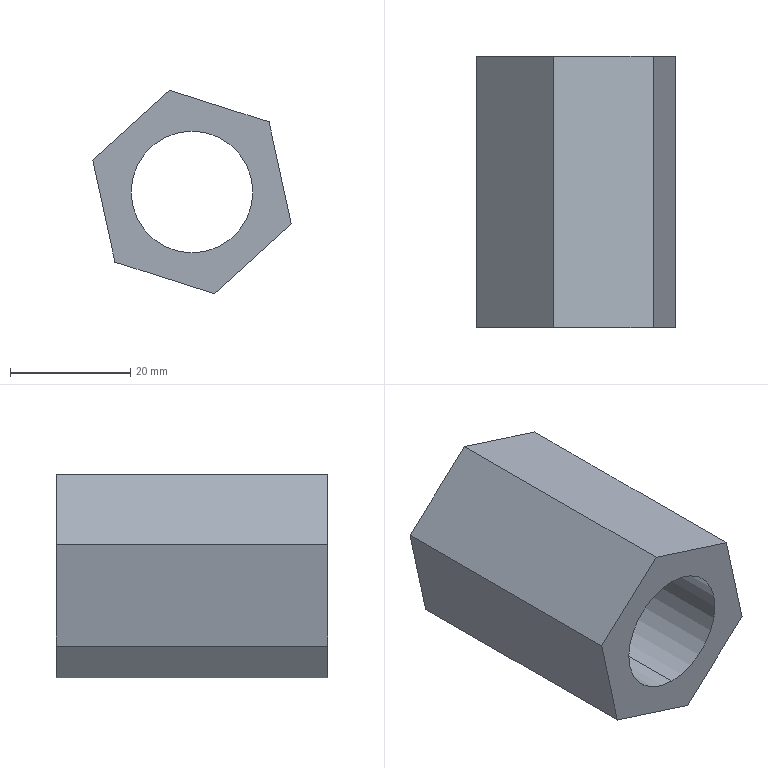Part | STEP file | 1 solid | 10 faces | box 32.935 x 45 x 33.783 mm | volume 20505 mm3 | plane 8 | cylinder 2 | commonest cylinder face diameters 20.209 x2
STEP:
#1=CARTESIAN_POINT('',(0.,0.,0.));
#2=DIRECTION('',(0.,0.,1.));
#3=DIRECTION('',(1.,0.,0.));
#4=AXIS2_PLACEMENT_3D('',#1,#2,#3);
#5=CARTESIAN_POINT('',(340.649,189.014,256.211));
#6=VERTEX_POINT('',#5);
#7=CARTESIAN_POINT('',(340.649,234.014,256.211));
#8=VERTEX_POINT('',#7);
#9=CARTESIAN_POINT('',(340.649,189.014,256.211));
#10=DIRECTION('',(0.,1.,0.));
#11=VECTOR('',#10,1.);
#12=LINE('',#9,#11);
#13=CARTESIAN_POINT('',(340.649,189.014,246.106));
#14=DIRECTION('',(0.,1.,0.));
#15=DIRECTION('',(0.,0.,1.));
#16=AXIS2_PLACEMENT_3D('',#13,#14,#15);
#17=CYLINDRICAL_SURFACE('',#16,10.105);
#18=CARTESIAN_POINT('',(6.283,0.));
#19=DIRECTION('',(0.,1.));
#20=VECTOR('',#19,1.);
#21=LINE('',#18,#20);
#22=(GEOMETRIC_REPRESENTATION_CONTEXT(2)PARAMETRIC_REPRESENTATION_CONTEXT()REPRESENTATION_CONTEXT('',''));
#23=DEFINITIONAL_REPRESENTATION('',(#21),#22);
#24=PCURVE('',#17,#23);
#25=CARTESIAN_POINT('',(340.649,189.014,246.106));
#26=DIRECTION('',(0.,1.,0.));
#27=DIRECTION('',(0.,0.,1.));
#28=AXIS2_PLACEMENT_3D('',#25,#26,#27);
#29=CYLINDRICAL_SURFACE('',#28,10.105);
#30=CARTESIAN_POINT('',(0.,0.));
#31=DIRECTION('',(0.,1.));
#32=VECTOR('',#31,1.);
#33=LINE('',#30,#32);
#34=(GEOMETRIC_REPRESENTATION_CONTEXT(2)PARAMETRIC_REPRESENTATION_CONTEXT()REPRESENTATION_CONTEXT('',''));
#35=DEFINITIONAL_REPRESENTATION('',(#33),#34);
#36=PCURVE('',#29,#35);
#37=SURFACE_CURVE('',#12,(#24,#36),.PCURVE_S1.);
#38=EDGE_CURVE('',#6,#8,#37,.T.);
#39=ORIENTED_EDGE('',*,*,#38,.T.);
#40=CARTESIAN_POINT('',(340.649,234.014,236.001));
#41=VERTEX_POINT('',#40);
#42=CARTESIAN_POINT('',(340.649,234.014,246.106));
#43=DIRECTION('',(0.,-1.,0.));
#44=DIRECTION('',(0.,0.,-1.));
#45=AXIS2_PLACEMENT_3D('',#42,#43,#44);
#46=CIRCLE('',#45,10.105);
#47=CARTESIAN_POINT('',(9.425,45.));
#48=DIRECTION('',(-1.,0.));
#49=VECTOR('',#48,1.);
#50=LINE('',#47,#49);
#51=(GEOMETRIC_REPRESENTATION_CONTEXT(2)PARAMETRIC_REPRESENTATION_CONTEXT()REPRESENTATION_CONTEXT('',''));
#52=DEFINITIONAL_REPRESENTATION('',(#50),#51);
#53=PCURVE('',#17,#52);
#54=CARTESIAN_POINT('',(0.,234.014,0.));
#55=DIRECTION('',(0.,-1.,0.));
#56=DIRECTION('',(0.,0.,-1.));
#57=AXIS2_PLACEMENT_3D('',#54,#55,#56);
#58=PLANE('',#57);
#59=CARTESIAN_POINT('',(-246.106,340.649));
#60=DIRECTION('',(1.,0.));
#61=AXIS2_PLACEMENT_2D('',#59,#60);
#62=CIRCLE('',#61,10.105);
#63=(GEOMETRIC_REPRESENTATION_CONTEXT(2)PARAMETRIC_REPRESENTATION_CONTEXT()REPRESENTATION_CONTEXT('',''));
#64=DEFINITIONAL_REPRESENTATION('',(#62),#63);
#65=PCURVE('',#58,#64);
#66=SURFACE_CURVE('',#46,(#53,#65),.PCURVE_S1.);
#67=EDGE_CURVE('',#8,#41,#66,.T.);
#68=ORIENTED_EDGE('',*,*,#67,.T.);
#69=CARTESIAN_POINT('',(340.649,189.014,236.001));
#70=VERTEX_POINT('',#69);
#71=CARTESIAN_POINT('',(340.649,189.014,236.001));
#72=DIRECTION('',(0.,1.,0.));
#73=VECTOR('',#72,1.);
#74=LINE('',#71,#73);
#75=CARTESIAN_POINT('',(3.142,0.));
#76=DIRECTION('',(0.,1.));
#77=VECTOR('',#76,1.);
#78=LINE('',#75,#77);
#79=(GEOMETRIC_REPRESENTATION_CONTEXT(2)PARAMETRIC_REPRESENTATION_CONTEXT()REPRESENTATION_CONTEXT('',''));
#80=DEFINITIONAL_REPRESENTATION('',(#78),#79);
#81=PCURVE('',#17,#80);
#82=CARTESIAN_POINT('',(3.142,0.));
#83=DIRECTION('',(0.,1.));
#84=VECTOR('',#83,1.);
#85=LINE('',#82,#84);
#86=(GEOMETRIC_REPRESENTATION_CONTEXT(2)PARAMETRIC_REPRESENTATION_CONTEXT()REPRESENTATION_CONTEXT('',''));
#87=DEFINITIONAL_REPRESENTATION('',(#85),#86);
#88=PCURVE('',#29,#87);
#89=SURFACE_CURVE('',#74,(#81,#88),.PCURVE_S1.);
#90=EDGE_CURVE('',#70,#41,#89,.T.);
#91=ORIENTED_EDGE('',*,*,#90,.F.);
#92=CARTESIAN_POINT('',(340.649,189.014,246.106));
#93=DIRECTION('',(0.,-1.,0.));
#94=DIRECTION('',(0.,0.,-1.));
#95=AXIS2_PLACEMENT_3D('',#92,#93,#94);
#96=CIRCLE('',#95,10.105);
#97=CARTESIAN_POINT('',(9.425,0.));
#98=DIRECTION('',(-1.,0.));
#99=VECTOR('',#98,1.);
#100=LINE('',#97,#99);
#101=(GEOMETRIC_REPRESENTATION_CONTEXT(2)PARAMETRIC_REPRESENTATION_CONTEXT()REPRESENTATION_CONTEXT('',''));
#102=DEFINITIONAL_REPRESENTATION('',(#100),#101);
#103=PCURVE('',#17,#102);
#104=CARTESIAN_POINT('',(0.,189.014,0.));
#105=DIRECTION('',(0.,-1.,0.));
#106=DIRECTION('',(0.,0.,-1.));
#107=AXIS2_PLACEMENT_3D('',#104,#105,#106);
#108=PLANE('',#107);
#109=CARTESIAN_POINT('',(-246.106,340.649));
#110=DIRECTION('',(1.,0.));
#111=AXIS2_PLACEMENT_2D('',#109,#110);
#112=CIRCLE('',#111,10.105);
#113=(GEOMETRIC_REPRESENTATION_CONTEXT(2)PARAMETRIC_REPRESENTATION_CONTEXT()REPRESENTATION_CONTEXT('',''));
#114=DEFINITIONAL_REPRESENTATION('',(#112),#113);
#115=PCURVE('',#108,#114);
#116=SURFACE_CURVE('',#96,(#103,#115),.PCURVE_S1.);
#117=EDGE_CURVE('',#6,#70,#116,.T.);
#118=ORIENTED_EDGE('',*,*,#117,.F.);
#119=EDGE_LOOP('',(#39,#68,#91,#118));
#120=FACE_BOUND('',#119,.F.);
#121=ADVANCED_FACE('',(#120),#17,.F.);
#122=CARTESIAN_POINT('',(357.116,189.014,240.846));
#123=VERTEX_POINT('',#122);
#124=CARTESIAN_POINT('',(353.438,189.014,257.737));
#125=VERTEX_POINT('',#124);
#126=CARTESIAN_POINT('',(357.116,189.014,240.846));
#127=DIRECTION('',(-0.2128,0.,0.9771));
#128=VECTOR('',#127,1.);
#129=LINE('',#126,#128);
#130=CARTESIAN_POINT('',(-240.846,357.116));
#131=DIRECTION('',(-0.9771,-0.2128));
#132=VECTOR('',#131,1.);
#133=LINE('',#130,#132);
#134=(GEOMETRIC_REPRESENTATION_CONTEXT(2)PARAMETRIC_REPRESENTATION_CONTEXT()REPRESENTATION_CONTEXT('',''));
#135=DEFINITIONAL_REPRESENTATION('',(#133),#134);
#136=PCURVE('',#108,#135);
#137=CARTESIAN_POINT('',(357.116,189.014,240.846));
#138=DIRECTION('',(-0.9771,0.,-0.2128));
#139=DIRECTION('',(-0.2128,0.,0.9771));
#140=AXIS2_PLACEMENT_3D('',#137,#138,#139);
#141=PLANE('',#140);
#142=CARTESIAN_POINT('',(0.,0.));
#143=DIRECTION('',(1.,0.));
#144=VECTOR('',#143,1.);
#145=LINE('',#142,#144);
#146=(GEOMETRIC_REPRESENTATION_CONTEXT(2)PARAMETRIC_REPRESENTATION_CONTEXT()REPRESENTATION_CONTEXT('',''));
#147=DEFINITIONAL_REPRESENTATION('',(#145),#146);
#148=PCURVE('',#141,#147);
#149=SURFACE_CURVE('',#129,(#136,#148),.PCURVE_S1.);
#150=EDGE_CURVE('',#123,#125,#149,.T.);
#151=ORIENTED_EDGE('',*,*,#150,.T.);
#152=CARTESIAN_POINT('',(336.97,189.014,262.997));
#153=VERTEX_POINT('',#152);
#154=CARTESIAN_POINT('',(353.438,189.014,257.737));
#155=DIRECTION('',(-0.9526,0.,0.3043));
#156=VECTOR('',#155,1.);
#157=LINE('',#154,#156);
#158=CARTESIAN_POINT('',(-257.737,353.438));
#159=DIRECTION('',(-0.3043,-0.9526));
#160=VECTOR('',#159,1.);
#161=LINE('',#158,#160);
#162=(GEOMETRIC_REPRESENTATION_CONTEXT(2)PARAMETRIC_REPRESENTATION_CONTEXT()REPRESENTATION_CONTEXT('',''));
#163=DEFINITIONAL_REPRESENTATION('',(#161),#162);
#164=PCURVE('',#108,#163);
#165=CARTESIAN_POINT('',(353.438,189.014,257.737));
#166=DIRECTION('',(-0.3043,0.,-0.9526));
#167=DIRECTION('',(-0.9526,0.,0.3043));
#168=AXIS2_PLACEMENT_3D('',#165,#166,#167);
#169=PLANE('',#168);
#170=CARTESIAN_POINT('',(0.,0.));
#171=DIRECTION('',(1.,0.));
#172=VECTOR('',#171,1.);
#173=LINE('',#170,#172);
#174=(GEOMETRIC_REPRESENTATION_CONTEXT(2)PARAMETRIC_REPRESENTATION_CONTEXT()REPRESENTATION_CONTEXT('',''));
#175=DEFINITIONAL_REPRESENTATION('',(#173),#174);
#176=PCURVE('',#169,#175);
#177=SURFACE_CURVE('',#157,(#164,#176),.PCURVE_S1.);
#178=EDGE_CURVE('',#125,#153,#177,.T.);
#179=ORIENTED_EDGE('',*,*,#178,.T.);
#180=CARTESIAN_POINT('',(324.181,189.014,251.366));
#181=VERTEX_POINT('',#180);
#182=CARTESIAN_POINT('',(336.97,189.014,262.997));
#183=DIRECTION('',(-0.7398,0.,-0.6728));
#184=VECTOR('',#183,1.);
#185=LINE('',#182,#184);
#186=CARTESIAN_POINT('',(-262.997,336.97));
#187=DIRECTION('',(0.6728,-0.7398));
#188=VECTOR('',#187,1.);
#189=LINE('',#186,#188);
#190=(GEOMETRIC_REPRESENTATION_CONTEXT(2)PARAMETRIC_REPRESENTATION_CONTEXT()REPRESENTATION_CONTEXT('',''));
#191=DEFINITIONAL_REPRESENTATION('',(#189),#190);
#192=PCURVE('',#108,#191);
#193=CARTESIAN_POINT('',(336.97,189.014,262.997));
#194=DIRECTION('',(0.6728,0.,-0.7398));
#195=DIRECTION('',(-0.7398,0.,-0.6728));
#196=AXIS2_PLACEMENT_3D('',#193,#194,#195);
#197=PLANE('',#196);
#198=CARTESIAN_POINT('',(0.,0.));
#199=DIRECTION('',(1.,0.));
#200=VECTOR('',#199,1.);
#201=LINE('',#198,#200);
#202=(GEOMETRIC_REPRESENTATION_CONTEXT(2)PARAMETRIC_REPRESENTATION_CONTEXT()REPRESENTATION_CONTEXT('',''));
#203=DEFINITIONAL_REPRESENTATION('',(#201),#202);
#204=PCURVE('',#197,#203);
#205=SURFACE_CURVE('',#185,(#192,#204),.PCURVE_S1.);
#206=EDGE_CURVE('',#153,#181,#205,.T.);
#207=ORIENTED_EDGE('',*,*,#206,.T.);
#208=CARTESIAN_POINT('',(327.859,189.014,234.474));
#209=VERTEX_POINT('',#208);
#210=CARTESIAN_POINT('',(324.181,189.014,251.366));
#211=DIRECTION('',(0.2128,0.,-0.9771));
#212=VECTOR('',#211,1.);
#213=LINE('',#210,#212);
#214=CARTESIAN_POINT('',(-251.366,324.181));
#215=DIRECTION('',(0.9771,0.2128));
#216=VECTOR('',#215,1.);
#217=LINE('',#214,#216);
#218=(GEOMETRIC_REPRESENTATION_CONTEXT(2)PARAMETRIC_REPRESENTATION_CONTEXT()REPRESENTATION_CONTEXT('',''));
#219=DEFINITIONAL_REPRESENTATION('',(#217),#218);
#220=PCURVE('',#108,#219);
#221=CARTESIAN_POINT('',(324.181,189.014,251.366));
#222=DIRECTION('',(0.9771,0.,0.2128));
#223=DIRECTION('',(0.2128,0.,-0.9771));
#224=AXIS2_PLACEMENT_3D('',#221,#222,#223);
#225=PLANE('',#224);
#226=CARTESIAN_POINT('',(0.,0.));
#227=DIRECTION('',(1.,0.));
#228=VECTOR('',#227,1.);
#229=LINE('',#226,#228);
#230=(GEOMETRIC_REPRESENTATION_CONTEXT(2)PARAMETRIC_REPRESENTATION_CONTEXT()REPRESENTATION_CONTEXT('',''));
#231=DEFINITIONAL_REPRESENTATION('',(#229),#230);
#232=PCURVE('',#225,#231);
#233=SURFACE_CURVE('',#213,(#220,#232),.PCURVE_S1.);
#234=EDGE_CURVE('',#181,#209,#233,.T.);
#235=ORIENTED_EDGE('',*,*,#234,.T.);
#236=CARTESIAN_POINT('',(344.327,189.014,229.214));
#237=VERTEX_POINT('',#236);
#238=CARTESIAN_POINT('',(327.859,189.014,234.474));
#239=DIRECTION('',(0.9526,0.,-0.3043));
#240=VECTOR('',#239,1.);
#241=LINE('',#238,#240);
#242=CARTESIAN_POINT('',(-234.474,327.859));
#243=DIRECTION('',(0.3043,0.9526));
#244=VECTOR('',#243,1.);
#245=LINE('',#242,#244);
#246=(GEOMETRIC_REPRESENTATION_CONTEXT(2)PARAMETRIC_REPRESENTATION_CONTEXT()REPRESENTATION_CONTEXT('',''));
#247=DEFINITIONAL_REPRESENTATION('',(#245),#246);
#248=PCURVE('',#108,#247);
#249=CARTESIAN_POINT('',(327.859,189.014,234.474));
#250=DIRECTION('',(0.3043,0.,0.9526));
#251=DIRECTION('',(0.9526,0.,-0.3043));
#252=AXIS2_PLACEMENT_3D('',#249,#250,#251);
#253=PLANE('',#252);
#254=CARTESIAN_POINT('',(0.,0.));
#255=DIRECTION('',(1.,0.));
#256=VECTOR('',#255,1.);
#257=LINE('',#254,#256);
#258=(GEOMETRIC_REPRESENTATION_CONTEXT(2)PARAMETRIC_REPRESENTATION_CONTEXT()REPRESENTATION_CONTEXT('',''));
#259=DEFINITIONAL_REPRESENTATION('',(#257),#258);
#260=PCURVE('',#253,#259);
#261=SURFACE_CURVE('',#241,(#248,#260),.PCURVE_S1.);
#262=EDGE_CURVE('',#209,#237,#261,.T.);
#263=ORIENTED_EDGE('',*,*,#262,.T.);
#264=CARTESIAN_POINT('',(344.327,189.014,229.214));
#265=DIRECTION('',(0.7398,0.,0.6728));
#266=VECTOR('',#265,1.);
#267=LINE('',#264,#266);
#268=CARTESIAN_POINT('',(-229.214,344.327));
#269=DIRECTION('',(-0.6728,0.7398));
#270=VECTOR('',#269,1.);
#271=LINE('',#268,#270);
#272=(GEOMETRIC_REPRESENTATION_CONTEXT(2)PARAMETRIC_REPRESENTATION_CONTEXT()REPRESENTATION_CONTEXT('',''));
#273=DEFINITIONAL_REPRESENTATION('',(#271),#272);
#274=PCURVE('',#108,#273);
#275=CARTESIAN_POINT('',(344.327,189.014,229.214));
#276=DIRECTION('',(-0.6728,0.,0.7398));
#277=DIRECTION('',(0.7398,0.,0.6728));
#278=AXIS2_PLACEMENT_3D('',#275,#276,#277);
#279=PLANE('',#278);
#280=CARTESIAN_POINT('',(0.,0.));
#281=DIRECTION('',(1.,0.));
#282=VECTOR('',#281,1.);
#283=LINE('',#280,#282);
#284=(GEOMETRIC_REPRESENTATION_CONTEXT(2)PARAMETRIC_REPRESENTATION_CONTEXT()REPRESENTATION_CONTEXT('',''));
#285=DEFINITIONAL_REPRESENTATION('',(#283),#284);
#286=PCURVE('',#279,#285);
#287=SURFACE_CURVE('',#267,(#274,#286),.PCURVE_S1.);
#288=EDGE_CURVE('',#237,#123,#287,.T.);
#289=ORIENTED_EDGE('',*,*,#288,.T.);
#290=EDGE_LOOP('',(#151,#179,#207,#235,#263,#289));
#291=FACE_BOUND('',#290,.T.);
#292=ORIENTED_EDGE('',*,*,#117,.F.);
#293=CARTESIAN_POINT('',(340.649,189.014,246.106));
#294=DIRECTION('',(0.,-1.,0.));
#295=DIRECTION('',(0.,0.,-1.));
#296=AXIS2_PLACEMENT_3D('',#293,#294,#295);
#297=CIRCLE('',#296,10.105);
#298=CARTESIAN_POINT('',(-246.106,340.649));
#299=DIRECTION('',(1.,0.));
#300=AXIS2_PLACEMENT_2D('',#298,#299);
#301=CIRCLE('',#300,10.105);
#302=(GEOMETRIC_REPRESENTATION_CONTEXT(2)PARAMETRIC_REPRESENTATION_CONTEXT()REPRESENTATION_CONTEXT('',''));
#303=DEFINITIONAL_REPRESENTATION('',(#301),#302);
#304=PCURVE('',#108,#303);
#305=CARTESIAN_POINT('',(3.142,0.));
#306=DIRECTION('',(-1.,0.));
#307=VECTOR('',#306,1.);
#308=LINE('',#305,#307);
#309=(GEOMETRIC_REPRESENTATION_CONTEXT(2)PARAMETRIC_REPRESENTATION_CONTEXT()REPRESENTATION_CONTEXT('',''));
#310=DEFINITIONAL_REPRESENTATION('',(#308),#309);
#311=PCURVE('',#29,#310);
#312=SURFACE_CURVE('',#297,(#304,#311),.PCURVE_S1.);
#313=EDGE_CURVE('',#70,#6,#312,.T.);
#314=ORIENTED_EDGE('',*,*,#313,.F.);
#315=EDGE_LOOP('',(#292,#314));
#316=FACE_BOUND('',#315,.T.);
#317=ADVANCED_FACE('',(#291,#316),#108,.T.);
#318=CARTESIAN_POINT('',(357.116,234.014,240.846));
#319=VERTEX_POINT('',#318);
#320=CARTESIAN_POINT('',(353.438,234.014,257.737));
#321=VERTEX_POINT('',#320);
#322=CARTESIAN_POINT('',(357.116,234.014,240.846));
#323=DIRECTION('',(-0.2128,0.,0.9771));
#324=VECTOR('',#323,1.);
#325=LINE('',#322,#324);
#326=CARTESIAN_POINT('',(-240.846,357.116));
#327=DIRECTION('',(-0.9771,-0.2128));
#328=VECTOR('',#327,1.);
#329=LINE('',#326,#328);
#330=(GEOMETRIC_REPRESENTATION_CONTEXT(2)PARAMETRIC_REPRESENTATION_CONTEXT()REPRESENTATION_CONTEXT('',''));
#331=DEFINITIONAL_REPRESENTATION('',(#329),#330);
#332=PCURVE('',#58,#331);
#333=CARTESIAN_POINT('',(0.,45.));
#334=DIRECTION('',(1.,0.));
#335=VECTOR('',#334,1.);
#336=LINE('',#333,#335);
#337=(GEOMETRIC_REPRESENTATION_CONTEXT(2)PARAMETRIC_REPRESENTATION_CONTEXT()REPRESENTATION_CONTEXT('',''));
#338=DEFINITIONAL_REPRESENTATION('',(#336),#337);
#339=PCURVE('',#141,#338);
#340=SURFACE_CURVE('',#325,(#332,#339),.PCURVE_S1.);
#341=EDGE_CURVE('',#319,#321,#340,.T.);
#342=ORIENTED_EDGE('',*,*,#341,.F.);
#343=CARTESIAN_POINT('',(344.327,234.014,229.214));
#344=VERTEX_POINT('',#343);
#345=CARTESIAN_POINT('',(344.327,234.014,229.214));
#346=DIRECTION('',(0.7398,0.,0.6728));
#347=VECTOR('',#346,1.);
#348=LINE('',#345,#347);
#349=CARTESIAN_POINT('',(-229.214,344.327));
#350=DIRECTION('',(-0.6728,0.7398));
#351=VECTOR('',#350,1.);
#352=LINE('',#349,#351);
#353=(GEOMETRIC_REPRESENTATION_CONTEXT(2)PARAMETRIC_REPRESENTATION_CONTEXT()REPRESENTATION_CONTEXT('',''));
#354=DEFINITIONAL_REPRESENTATION('',(#352),#353);
#355=PCURVE('',#58,#354);
#356=CARTESIAN_POINT('',(0.,45.));
#357=DIRECTION('',(1.,0.));
#358=VECTOR('',#357,1.);
#359=LINE('',#356,#358);
#360=(GEOMETRIC_REPRESENTATION_CONTEXT(2)PARAMETRIC_REPRESENTATION_CONTEXT()REPRESENTATION_CONTEXT('',''));
#361=DEFINITIONAL_REPRESENTATION('',(#359),#360);
#362=PCURVE('',#279,#361);
#363=SURFACE_CURVE('',#348,(#355,#362),.PCURVE_S1.);
#364=EDGE_CURVE('',#344,#319,#363,.T.);
#365=ORIENTED_EDGE('',*,*,#364,.F.);
#366=CARTESIAN_POINT('',(327.859,234.014,234.474));
#367=VERTEX_POINT('',#366);
#368=CARTESIAN_POINT('',(327.859,234.014,234.474));
#369=DIRECTION('',(0.9526,0.,-0.3043));
#370=VECTOR('',#369,1.);
#371=LINE('',#368,#370);
#372=CARTESIAN_POINT('',(-234.474,327.859));
#373=DIRECTION('',(0.3043,0.9526));
#374=VECTOR('',#373,1.);
#375=LINE('',#372,#374);
#376=(GEOMETRIC_REPRESENTATION_CONTEXT(2)PARAMETRIC_REPRESENTATION_CONTEXT()REPRESENTATION_CONTEXT('',''));
#377=DEFINITIONAL_REPRESENTATION('',(#375),#376);
#378=PCURVE('',#58,#377);
#379=CARTESIAN_POINT('',(0.,45.));
#380=DIRECTION('',(1.,0.));
#381=VECTOR('',#380,1.);
#382=LINE('',#379,#381);
#383=(GEOMETRIC_REPRESENTATION_CONTEXT(2)PARAMETRIC_REPRESENTATION_CONTEXT()REPRESENTATION_CONTEXT('',''));
#384=DEFINITIONAL_REPRESENTATION('',(#382),#383);
#385=PCURVE('',#253,#384);
#386=SURFACE_CURVE('',#371,(#378,#385),.PCURVE_S1.);
#387=EDGE_CURVE('',#367,#344,#386,.T.);
#388=ORIENTED_EDGE('',*,*,#387,.F.);
#389=CARTESIAN_POINT('',(324.181,234.014,251.366));
#390=VERTEX_POINT('',#389);
#391=CARTESIAN_POINT('',(324.181,234.014,251.366));
#392=DIRECTION('',(0.2128,0.,-0.9771));
#393=VECTOR('',#392,1.);
#394=LINE('',#391,#393);
#395=CARTESIAN_POINT('',(-251.366,324.181));
#396=DIRECTION('',(0.9771,0.2128));
#397=VECTOR('',#396,1.);
#398=LINE('',#395,#397);
#399=(GEOMETRIC_REPRESENTATION_CONTEXT(2)PARAMETRIC_REPRESENTATION_CONTEXT()REPRESENTATION_CONTEXT('',''));
#400=DEFINITIONAL_REPRESENTATION('',(#398),#399);
#401=PCURVE('',#58,#400);
#402=CARTESIAN_POINT('',(0.,45.));
#403=DIRECTION('',(1.,0.));
#404=VECTOR('',#403,1.);
#405=LINE('',#402,#404);
#406=(GEOMETRIC_REPRESENTATION_CONTEXT(2)PARAMETRIC_REPRESENTATION_CONTEXT()REPRESENTATION_CONTEXT('',''));
#407=DEFINITIONAL_REPRESENTATION('',(#405),#406);
#408=PCURVE('',#225,#407);
#409=SURFACE_CURVE('',#394,(#401,#408),.PCURVE_S1.);
#410=EDGE_CURVE('',#390,#367,#409,.T.);
#411=ORIENTED_EDGE('',*,*,#410,.F.);
#412=CARTESIAN_POINT('',(336.97,234.014,262.997));
#413=VERTEX_POINT('',#412);
#414=CARTESIAN_POINT('',(336.97,234.014,262.997));
#415=DIRECTION('',(-0.7398,0.,-0.6728));
#416=VECTOR('',#415,1.);
#417=LINE('',#414,#416);
#418=CARTESIAN_POINT('',(-262.997,336.97));
#419=DIRECTION('',(0.6728,-0.7398));
#420=VECTOR('',#419,1.);
#421=LINE('',#418,#420);
#422=(GEOMETRIC_REPRESENTATION_CONTEXT(2)PARAMETRIC_REPRESENTATION_CONTEXT()REPRESENTATION_CONTEXT('',''));
#423=DEFINITIONAL_REPRESENTATION('',(#421),#422);
#424=PCURVE('',#58,#423);
#425=CARTESIAN_POINT('',(0.,45.));
#426=DIRECTION('',(1.,0.));
#427=VECTOR('',#426,1.);
#428=LINE('',#425,#427);
#429=(GEOMETRIC_REPRESENTATION_CONTEXT(2)PARAMETRIC_REPRESENTATION_CONTEXT()REPRESENTATION_CONTEXT('',''));
#430=DEFINITIONAL_REPRESENTATION('',(#428),#429);
#431=PCURVE('',#197,#430);
#432=SURFACE_CURVE('',#417,(#424,#431),.PCURVE_S1.);
#433=EDGE_CURVE('',#413,#390,#432,.T.);
#434=ORIENTED_EDGE('',*,*,#433,.F.);
#435=CARTESIAN_POINT('',(353.438,234.014,257.737));
#436=DIRECTION('',(-0.9526,0.,0.3043));
#437=VECTOR('',#436,1.);
#438=LINE('',#435,#437);
#439=CARTESIAN_POINT('',(-257.737,353.438));
#440=DIRECTION('',(-0.3043,-0.9526));
#441=VECTOR('',#440,1.);
#442=LINE('',#439,#441);
#443=(GEOMETRIC_REPRESENTATION_CONTEXT(2)PARAMETRIC_REPRESENTATION_CONTEXT()REPRESENTATION_CONTEXT('',''));
#444=DEFINITIONAL_REPRESENTATION('',(#442),#443);
#445=PCURVE('',#58,#444);
#446=CARTESIAN_POINT('',(0.,45.));
#447=DIRECTION('',(1.,0.));
#448=VECTOR('',#447,1.);
#449=LINE('',#446,#448);
#450=(GEOMETRIC_REPRESENTATION_CONTEXT(2)PARAMETRIC_REPRESENTATION_CONTEXT()REPRESENTATION_CONTEXT('',''));
#451=DEFINITIONAL_REPRESENTATION('',(#449),#450);
#452=PCURVE('',#169,#451);
#453=SURFACE_CURVE('',#438,(#445,#452),.PCURVE_S1.);
#454=EDGE_CURVE('',#321,#413,#453,.T.);
#455=ORIENTED_EDGE('',*,*,#454,.F.);
#456=EDGE_LOOP('',(#342,#365,#388,#411,#434,#455));
#457=FACE_BOUND('',#456,.T.);
#458=ORIENTED_EDGE('',*,*,#67,.T.);
#459=CARTESIAN_POINT('',(340.649,234.014,246.106));
#460=DIRECTION('',(0.,-1.,0.));
#461=DIRECTION('',(0.,0.,-1.));
#462=AXIS2_PLACEMENT_3D('',#459,#460,#461);
#463=CIRCLE('',#462,10.105);
#464=CARTESIAN_POINT('',(-246.106,340.649));
#465=DIRECTION('',(1.,0.));
#466=AXIS2_PLACEMENT_2D('',#464,#465);
#467=CIRCLE('',#466,10.105);
#468=(GEOMETRIC_REPRESENTATION_CONTEXT(2)PARAMETRIC_REPRESENTATION_CONTEXT()REPRESENTATION_CONTEXT('',''));
#469=DEFINITIONAL_REPRESENTATION('',(#467),#468);
#470=PCURVE('',#58,#469);
#471=CARTESIAN_POINT('',(3.142,45.));
#472=DIRECTION('',(-1.,0.));
#473=VECTOR('',#472,1.);
#474=LINE('',#471,#473);
#475=(GEOMETRIC_REPRESENTATION_CONTEXT(2)PARAMETRIC_REPRESENTATION_CONTEXT()REPRESENTATION_CONTEXT('',''));
#476=DEFINITIONAL_REPRESENTATION('',(#474),#475);
#477=PCURVE('',#29,#476);
#478=SURFACE_CURVE('',#463,(#470,#477),.PCURVE_S1.);
#479=EDGE_CURVE('',#41,#8,#478,.T.);
#480=ORIENTED_EDGE('',*,*,#479,.T.);
#481=EDGE_LOOP('',(#458,#480));
#482=FACE_BOUND('',#481,.T.);
#483=ADVANCED_FACE('',(#457,#482),#58,.F.);
#484=ORIENTED_EDGE('',*,*,#341,.T.);
#485=CARTESIAN_POINT('',(353.438,189.014,257.737));
#486=DIRECTION('',(0.,1.,0.));
#487=VECTOR('',#486,1.);
#488=LINE('',#485,#487);
#489=CARTESIAN_POINT('',(17.287,0.));
#490=DIRECTION('',(0.,1.));
#491=VECTOR('',#490,1.);
#492=LINE('',#489,#491);
#493=(GEOMETRIC_REPRESENTATION_CONTEXT(2)PARAMETRIC_REPRESENTATION_CONTEXT()REPRESENTATION_CONTEXT('',''));
#494=DEFINITIONAL_REPRESENTATION('',(#492),#493);
#495=PCURVE('',#141,#494);
#496=CARTESIAN_POINT('',(0.,0.));
#497=DIRECTION('',(0.,1.));
#498=VECTOR('',#497,1.);
#499=LINE('',#496,#498);
#500=(GEOMETRIC_REPRESENTATION_CONTEXT(2)PARAMETRIC_REPRESENTATION_CONTEXT()REPRESENTATION_CONTEXT('',''));
#501=DEFINITIONAL_REPRESENTATION('',(#499),#500);
#502=PCURVE('',#169,#501);
#503=SURFACE_CURVE('',#488,(#495,#502),.PCURVE_S1.);
#504=EDGE_CURVE('',#125,#321,#503,.T.);
#505=ORIENTED_EDGE('',*,*,#504,.F.);
#506=ORIENTED_EDGE('',*,*,#150,.F.);
#507=CARTESIAN_POINT('',(357.116,189.014,240.846));
#508=DIRECTION('',(0.,1.,0.));
#509=VECTOR('',#508,1.);
#510=LINE('',#507,#509);
#511=CARTESIAN_POINT('',(0.,0.));
#512=DIRECTION('',(0.,1.));
#513=VECTOR('',#512,1.);
#514=LINE('',#511,#513);
#515=(GEOMETRIC_REPRESENTATION_CONTEXT(2)PARAMETRIC_REPRESENTATION_CONTEXT()REPRESENTATION_CONTEXT('',''));
#516=DEFINITIONAL_REPRESENTATION('',(#514),#515);
#517=PCURVE('',#141,#516);
#518=CARTESIAN_POINT('',(17.287,0.));
#519=DIRECTION('',(0.,1.));
#520=VECTOR('',#519,1.);
#521=LINE('',#518,#520);
#522=(GEOMETRIC_REPRESENTATION_CONTEXT(2)PARAMETRIC_REPRESENTATION_CONTEXT()REPRESENTATION_CONTEXT('',''));
#523=DEFINITIONAL_REPRESENTATION('',(#521),#522);
#524=PCURVE('',#279,#523);
#525=SURFACE_CURVE('',#510,(#517,#524),.PCURVE_S1.);
#526=EDGE_CURVE('',#123,#319,#525,.T.);
#527=ORIENTED_EDGE('',*,*,#526,.T.);
#528=EDGE_LOOP('',(#484,#505,#506,#527));
#529=FACE_BOUND('',#528,.T.);
#530=ADVANCED_FACE('',(#529),#141,.F.);
#531=ORIENTED_EDGE('',*,*,#454,.T.);
#532=CARTESIAN_POINT('',(336.97,189.014,262.997));
#533=DIRECTION('',(0.,1.,0.));
#534=VECTOR('',#533,1.);
#535=LINE('',#532,#534);
#536=CARTESIAN_POINT('',(17.287,0.));
#537=DIRECTION('',(0.,1.));
#538=VECTOR('',#537,1.);
#539=LINE('',#536,#538);
#540=(GEOMETRIC_REPRESENTATION_CONTEXT(2)PARAMETRIC_REPRESENTATION_CONTEXT()REPRESENTATION_CONTEXT('',''));
#541=DEFINITIONAL_REPRESENTATION('',(#539),#540);
#542=PCURVE('',#169,#541);
#543=CARTESIAN_POINT('',(0.,0.));
#544=DIRECTION('',(0.,1.));
#545=VECTOR('',#544,1.);
#546=LINE('',#543,#545);
#547=(GEOMETRIC_REPRESENTATION_CONTEXT(2)PARAMETRIC_REPRESENTATION_CONTEXT()REPRESENTATION_CONTEXT('',''));
#548=DEFINITIONAL_REPRESENTATION('',(#546),#547);
#549=PCURVE('',#197,#548);
#550=SURFACE_CURVE('',#535,(#542,#549),.PCURVE_S1.);
#551=EDGE_CURVE('',#153,#413,#550,.T.);
#552=ORIENTED_EDGE('',*,*,#551,.F.);
#553=ORIENTED_EDGE('',*,*,#178,.F.);
#554=ORIENTED_EDGE('',*,*,#504,.T.);
#555=EDGE_LOOP('',(#531,#552,#553,#554));
#556=FACE_BOUND('',#555,.T.);
#557=ADVANCED_FACE('',(#556),#169,.F.);
#558=ORIENTED_EDGE('',*,*,#433,.T.);
#559=CARTESIAN_POINT('',(324.181,189.014,251.366));
#560=DIRECTION('',(0.,1.,0.));
#561=VECTOR('',#560,1.);
#562=LINE('',#559,#561);
#563=CARTESIAN_POINT('',(17.287,0.));
#564=DIRECTION('',(0.,1.));
#565=VECTOR('',#564,1.);
#566=LINE('',#563,#565);
#567=(GEOMETRIC_REPRESENTATION_CONTEXT(2)PARAMETRIC_REPRESENTATION_CONTEXT()REPRESENTATION_CONTEXT('',''));
#568=DEFINITIONAL_REPRESENTATION('',(#566),#567);
#569=PCURVE('',#197,#568);
#570=CARTESIAN_POINT('',(0.,0.));
#571=DIRECTION('',(0.,1.));
#572=VECTOR('',#571,1.);
#573=LINE('',#570,#572);
#574=(GEOMETRIC_REPRESENTATION_CONTEXT(2)PARAMETRIC_REPRESENTATION_CONTEXT()REPRESENTATION_CONTEXT('',''));
#575=DEFINITIONAL_REPRESENTATION('',(#573),#574);
#576=PCURVE('',#225,#575);
#577=SURFACE_CURVE('',#562,(#569,#576),.PCURVE_S1.);
#578=EDGE_CURVE('',#181,#390,#577,.T.);
#579=ORIENTED_EDGE('',*,*,#578,.F.);
#580=ORIENTED_EDGE('',*,*,#206,.F.);
#581=ORIENTED_EDGE('',*,*,#551,.T.);
#582=EDGE_LOOP('',(#558,#579,#580,#581));
#583=FACE_BOUND('',#582,.T.);
#584=ADVANCED_FACE('',(#583),#197,.F.);
#585=ORIENTED_EDGE('',*,*,#410,.T.);
#586=CARTESIAN_POINT('',(327.859,189.014,234.474));
#587=DIRECTION('',(0.,1.,0.));
#588=VECTOR('',#587,1.);
#589=LINE('',#586,#588);
#590=CARTESIAN_POINT('',(17.287,0.));
#591=DIRECTION('',(0.,1.));
#592=VECTOR('',#591,1.);
#593=LINE('',#590,#592);
#594=(GEOMETRIC_REPRESENTATION_CONTEXT(2)PARAMETRIC_REPRESENTATION_CONTEXT()REPRESENTATION_CONTEXT('',''));
#595=DEFINITIONAL_REPRESENTATION('',(#593),#594);
#596=PCURVE('',#225,#595);
#597=CARTESIAN_POINT('',(0.,0.));
#598=DIRECTION('',(0.,1.));
#599=VECTOR('',#598,1.);
#600=LINE('',#597,#599);
#601=(GEOMETRIC_REPRESENTATION_CONTEXT(2)PARAMETRIC_REPRESENTATION_CONTEXT()REPRESENTATION_CONTEXT('',''));
#602=DEFINITIONAL_REPRESENTATION('',(#600),#601);
#603=PCURVE('',#253,#602);
#604=SURFACE_CURVE('',#589,(#596,#603),.PCURVE_S1.);
#605=EDGE_CURVE('',#209,#367,#604,.T.);
#606=ORIENTED_EDGE('',*,*,#605,.F.);
#607=ORIENTED_EDGE('',*,*,#234,.F.);
#608=ORIENTED_EDGE('',*,*,#578,.T.);
#609=EDGE_LOOP('',(#585,#606,#607,#608));
#610=FACE_BOUND('',#609,.T.);
#611=ADVANCED_FACE('',(#610),#225,.F.);
#612=ORIENTED_EDGE('',*,*,#387,.T.);
#613=CARTESIAN_POINT('',(344.327,189.014,229.214));
#614=DIRECTION('',(0.,1.,0.));
#615=VECTOR('',#614,1.);
#616=LINE('',#613,#615);
#617=CARTESIAN_POINT('',(17.287,0.));
#618=DIRECTION('',(0.,1.));
#619=VECTOR('',#618,1.);
#620=LINE('',#617,#619);
#621=(GEOMETRIC_REPRESENTATION_CONTEXT(2)PARAMETRIC_REPRESENTATION_CONTEXT()REPRESENTATION_CONTEXT('',''));
#622=DEFINITIONAL_REPRESENTATION('',(#620),#621);
#623=PCURVE('',#253,#622);
#624=CARTESIAN_POINT('',(0.,0.));
#625=DIRECTION('',(0.,1.));
#626=VECTOR('',#625,1.);
#627=LINE('',#624,#626);
#628=(GEOMETRIC_REPRESENTATION_CONTEXT(2)PARAMETRIC_REPRESENTATION_CONTEXT()REPRESENTATION_CONTEXT('',''));
#629=DEFINITIONAL_REPRESENTATION('',(#627),#628);
#630=PCURVE('',#279,#629);
#631=SURFACE_CURVE('',#616,(#623,#630),.PCURVE_S1.);
#632=EDGE_CURVE('',#237,#344,#631,.T.);
#633=ORIENTED_EDGE('',*,*,#632,.F.);
#634=ORIENTED_EDGE('',*,*,#262,.F.);
#635=ORIENTED_EDGE('',*,*,#605,.T.);
#636=EDGE_LOOP('',(#612,#633,#634,#635));
#637=FACE_BOUND('',#636,.T.);
#638=ADVANCED_FACE('',(#637),#253,.F.);
#639=ORIENTED_EDGE('',*,*,#364,.T.);
#640=ORIENTED_EDGE('',*,*,#526,.F.);
#641=ORIENTED_EDGE('',*,*,#288,.F.);
#642=ORIENTED_EDGE('',*,*,#632,.T.);
#643=EDGE_LOOP('',(#639,#640,#641,#642));
#644=FACE_BOUND('',#643,.T.);
#645=ADVANCED_FACE('',(#644),#279,.F.);
#646=ORIENTED_EDGE('',*,*,#479,.T.);
#647=ORIENTED_EDGE('',*,*,#38,.F.);
#648=ORIENTED_EDGE('',*,*,#313,.F.);
#649=ORIENTED_EDGE('',*,*,#90,.T.);
#650=EDGE_LOOP('',(#646,#647,#648,#649));
#651=FACE_BOUND('',#650,.F.);
#652=ADVANCED_FACE('',(#651),#29,.F.);
#653=CLOSED_SHELL('',(#121,#317,#483,#530,#557,#584,#611,#638,#645,#652));
#654=MANIFOLD_SOLID_BREP('',#653);
#655=(LENGTH_UNIT()NAMED_UNIT(*)SI_UNIT(.MILLI.,.METRE.));
#656=UNCERTAINTY_MEASURE_WITH_UNIT(LENGTH_MEASURE(0.0000001),#655,'','');
#657=(NAMED_UNIT(*)PLANE_ANGLE_UNIT()SI_UNIT($,.RADIAN.));
#658=(NAMED_UNIT(*)SI_UNIT($,.STERADIAN.)SOLID_ANGLE_UNIT());
#659=(GEOMETRIC_REPRESENTATION_CONTEXT(3)GLOBAL_UNCERTAINTY_ASSIGNED_CONTEXT((#656))GLOBAL_UNIT_ASSIGNED_CONTEXT((#655,#657,#658))REPRESENTATION_CONTEXT('',''));
#660=ADVANCED_BREP_SHAPE_REPRESENTATION('',(#4,#654),#659);